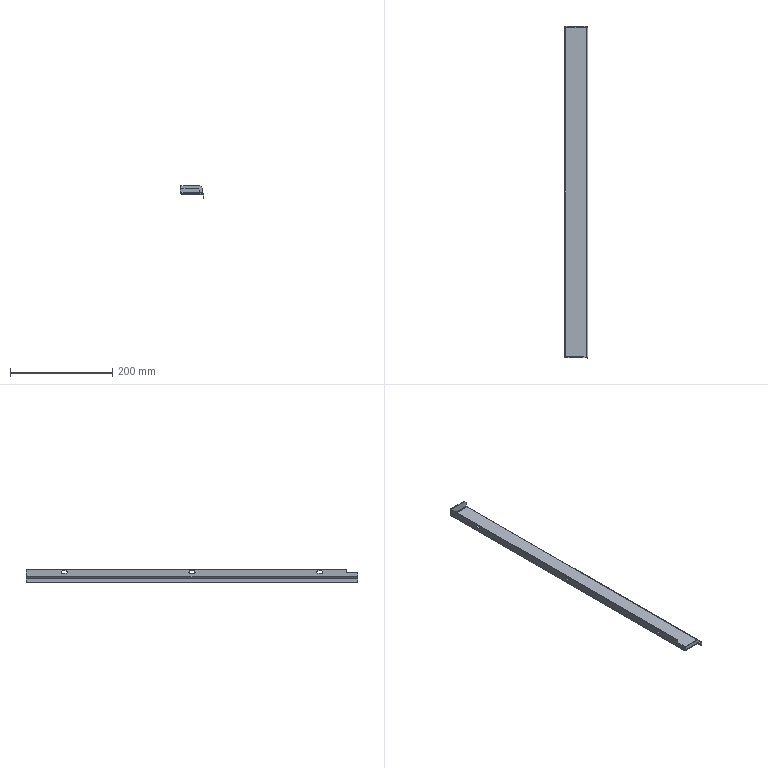Part | NX | features solid 2 | 1 solid | 58 faces | box 46.5 x 650 x 25 mm | volume 67197 mm3 | plane 44 | cylinder 14 | commonest cylinder face diameters 5 x6 3 x4 6 x4